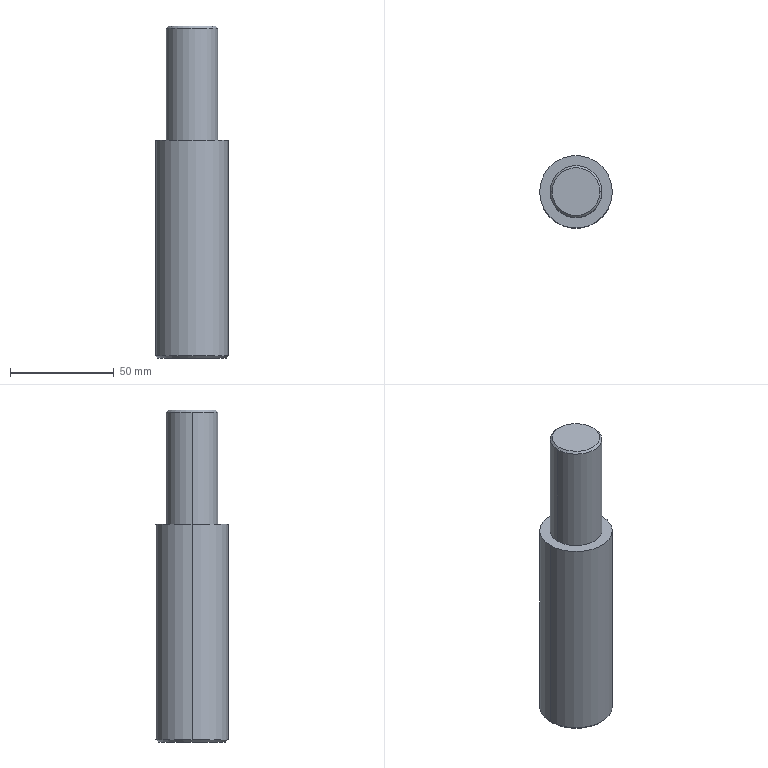Part | SolidWorks | features Chamfer 1, Extrusion 1, ICE 1 | 1 solid | 11 faces | box 35 x 35 x 160 mm | volume 127928 mm3 | cone 4 | cylinder 4 | plane 3 | commonest cylinder face diameters 25 x2 35 x2
STEP:
#1=CARTESIAN_POINT('',(11.5,0.,160.));
#2=VERTEX_POINT('',#1);
#3=CARTESIAN_POINT('',(-11.5,0.,160.));
#4=VERTEX_POINT('',#3);
#5=CARTESIAN_POINT('',(0.,0.,160.));
#6=DIRECTION('',(0.,0.,1.));
#7=DIRECTION('',(1.,0.,0.));
#8=AXIS2_PLACEMENT_3D('',#5,#6,#7);
#9=CIRCLE('',#8,11.5);
#10=EDGE_CURVE('',#2,#4,#9,.T.);
#11=ORIENTED_EDGE('',*,*,#10,.F.);
#12=CARTESIAN_POINT('',(12.5,0.,159.));
#13=VERTEX_POINT('',#12);
#14=CARTESIAN_POINT('',(11.5,0.,160.));
#15=DIRECTION('',(0.7071,0.,-0.7071));
#16=VECTOR('',#15,1000.);
#17=LINE('',#14,#16);
#18=EDGE_CURVE('',#2,#13,#17,.T.);
#19=ORIENTED_EDGE('',*,*,#18,.T.);
#20=CARTESIAN_POINT('',(-12.5,0.,159.));
#21=VERTEX_POINT('',#20);
#22=CARTESIAN_POINT('',(0.,0.,159.));
#23=DIRECTION('',(0.,0.,-1.));
#24=DIRECTION('',(1.,0.,0.));
#25=AXIS2_PLACEMENT_3D('',#22,#23,#24);
#26=CIRCLE('',#25,12.5);
#27=EDGE_CURVE('',#21,#13,#26,.T.);
#28=ORIENTED_EDGE('',*,*,#27,.F.);
#29=CARTESIAN_POINT('',(-11.5,0.,160.));
#30=DIRECTION('',(-0.7071,0.,-0.7071));
#31=VECTOR('',#30,1000.);
#32=LINE('',#29,#31);
#33=EDGE_CURVE('',#4,#21,#32,.T.);
#34=ORIENTED_EDGE('',*,*,#33,.F.);
#35=EDGE_LOOP('',(#11,#19,#28,#34));
#36=FACE_OUTER_BOUND('',#35,.T.);
#37=CARTESIAN_POINT('',(0.,0.,160.));
#38=DIRECTION('',(0.,0.,-1.));
#39=DIRECTION('',(-1.,0.,0.));
#40=AXIS2_PLACEMENT_3D('',#37,#38,#39);
#41=CONICAL_SURFACE('',#40,11.5,0.7854);
#42=ADVANCED_FACE('',(#36),#41,.T.);
#43=CARTESIAN_POINT('',(-16.5,0.,0.));
#44=VERTEX_POINT('',#43);
#45=CARTESIAN_POINT('',(16.5,0.,0.));
#46=VERTEX_POINT('',#45);
#47=CARTESIAN_POINT('',(0.,0.,0.));
#48=DIRECTION('',(0.,0.,-1.));
#49=DIRECTION('',(1.,0.,0.));
#50=AXIS2_PLACEMENT_3D('',#47,#48,#49);
#51=CIRCLE('',#50,16.5);
#52=EDGE_CURVE('',#44,#46,#51,.T.);
#53=ORIENTED_EDGE('',*,*,#52,.F.);
#54=CARTESIAN_POINT('',(-17.5,0.,1.));
#55=VERTEX_POINT('',#54);
#56=CARTESIAN_POINT('',(-17.5,0.,1.));
#57=DIRECTION('',(-0.7071,0.,0.7071));
#58=VECTOR('',#57,1000.);
#59=LINE('',#56,#58);
#60=EDGE_CURVE('',#44,#55,#59,.T.);
#61=ORIENTED_EDGE('',*,*,#60,.T.);
#62=CARTESIAN_POINT('',(17.5,0.,1.));
#63=VERTEX_POINT('',#62);
#64=CARTESIAN_POINT('',(0.,0.,1.));
#65=DIRECTION('',(0.,0.,1.));
#66=DIRECTION('',(1.,0.,0.));
#67=AXIS2_PLACEMENT_3D('',#64,#65,#66);
#68=CIRCLE('',#67,17.5);
#69=EDGE_CURVE('',#63,#55,#68,.T.);
#70=ORIENTED_EDGE('',*,*,#69,.F.);
#71=CARTESIAN_POINT('',(17.5,0.,1.));
#72=DIRECTION('',(0.7071,0.,0.7071));
#73=VECTOR('',#72,1000.);
#74=LINE('',#71,#73);
#75=EDGE_CURVE('',#46,#63,#74,.T.);
#76=ORIENTED_EDGE('',*,*,#75,.F.);
#77=EDGE_LOOP('',(#53,#61,#70,#76));
#78=FACE_OUTER_BOUND('',#77,.T.);
#79=CARTESIAN_POINT('',(0.,0.,1.));
#80=DIRECTION('',(0.,0.,1.));
#81=DIRECTION('',(1.,0.,0.));
#82=AXIS2_PLACEMENT_3D('',#79,#80,#81);
#83=CONICAL_SURFACE('',#82,17.5,0.7854);
#84=ADVANCED_FACE('',(#78),#83,.T.);
#85=ORIENTED_EDGE('',*,*,#27,.T.);
#86=CARTESIAN_POINT('',(12.5,0.,105.));
#87=VERTEX_POINT('',#86);
#88=CARTESIAN_POINT('',(12.5,0.,160.));
#89=DIRECTION('',(0.,0.,-1.));
#90=VECTOR('',#89,1000.);
#91=LINE('',#88,#90);
#92=EDGE_CURVE('',#13,#87,#91,.T.);
#93=ORIENTED_EDGE('',*,*,#92,.T.);
#94=CARTESIAN_POINT('',(-12.5,0.,105.));
#95=VERTEX_POINT('',#94);
#96=CARTESIAN_POINT('',(0.,0.,105.));
#97=DIRECTION('',(0.,0.,1.));
#98=DIRECTION('',(1.,0.,0.));
#99=AXIS2_PLACEMENT_3D('',#96,#97,#98);
#100=CIRCLE('',#99,12.5);
#101=EDGE_CURVE('',#87,#95,#100,.T.);
#102=ORIENTED_EDGE('',*,*,#101,.T.);
#103=CARTESIAN_POINT('',(-12.5,0.,160.));
#104=DIRECTION('',(0.,0.,-1.));
#105=VECTOR('',#104,1000.);
#106=LINE('',#103,#105);
#107=EDGE_CURVE('',#21,#95,#106,.T.);
#108=ORIENTED_EDGE('',*,*,#107,.F.);
#109=EDGE_LOOP('',(#85,#93,#102,#108));
#110=FACE_OUTER_BOUND('',#109,.T.);
#111=CARTESIAN_POINT('',(0.,0.,160.));
#112=DIRECTION('',(0.,0.,-1.));
#113=DIRECTION('',(-1.,0.,0.));
#114=AXIS2_PLACEMENT_3D('',#111,#112,#113);
#115=CYLINDRICAL_SURFACE('',#114,12.5);
#116=ADVANCED_FACE('',(#110),#115,.T.);
#117=CARTESIAN_POINT('',(17.5,0.,105.));
#118=VERTEX_POINT('',#117);
#119=CARTESIAN_POINT('',(-17.5,0.,105.));
#120=VERTEX_POINT('',#119);
#121=CARTESIAN_POINT('',(0.,0.,105.));
#122=DIRECTION('',(0.,0.,1.));
#123=DIRECTION('',(1.,0.,0.));
#124=AXIS2_PLACEMENT_3D('',#121,#122,#123);
#125=CIRCLE('',#124,17.5);
#126=EDGE_CURVE('',#118,#120,#125,.T.);
#127=ORIENTED_EDGE('',*,*,#126,.F.);
#128=CARTESIAN_POINT('',(17.5,0.,105.));
#129=DIRECTION('',(0.,0.,-1.));
#130=VECTOR('',#129,1000.);
#131=LINE('',#128,#130);
#132=EDGE_CURVE('',#118,#63,#131,.T.);
#133=ORIENTED_EDGE('',*,*,#132,.T.);
#134=ORIENTED_EDGE('',*,*,#69,.T.);
#135=CARTESIAN_POINT('',(-17.5,0.,105.));
#136=DIRECTION('',(0.,0.,-1.));
#137=VECTOR('',#136,1000.);
#138=LINE('',#135,#137);
#139=EDGE_CURVE('',#120,#55,#138,.T.);
#140=ORIENTED_EDGE('',*,*,#139,.F.);
#141=EDGE_LOOP('',(#127,#133,#134,#140));
#142=FACE_OUTER_BOUND('',#141,.T.);
#143=CARTESIAN_POINT('',(0.,0.,105.));
#144=DIRECTION('',(0.,0.,-1.));
#145=DIRECTION('',(-1.,0.,0.));
#146=AXIS2_PLACEMENT_3D('',#143,#144,#145);
#147=CYLINDRICAL_SURFACE('',#146,17.5);
#148=ADVANCED_FACE('',(#142),#147,.T.);
#149=ORIENTED_EDGE('',*,*,#132,.F.);
#150=CARTESIAN_POINT('',(0.,0.,105.));
#151=DIRECTION('',(0.,0.,1.));
#152=DIRECTION('',(1.,0.,0.));
#153=AXIS2_PLACEMENT_3D('',#150,#151,#152);
#154=CIRCLE('',#153,17.5);
#155=EDGE_CURVE('',#120,#118,#154,.T.);
#156=ORIENTED_EDGE('',*,*,#155,.F.);
#157=ORIENTED_EDGE('',*,*,#139,.T.);
#158=CARTESIAN_POINT('',(0.,0.,1.));
#159=DIRECTION('',(0.,0.,1.));
#160=DIRECTION('',(1.,0.,0.));
#161=AXIS2_PLACEMENT_3D('',#158,#159,#160);
#162=CIRCLE('',#161,17.5);
#163=EDGE_CURVE('',#55,#63,#162,.T.);
#164=ORIENTED_EDGE('',*,*,#163,.T.);
#165=EDGE_LOOP('',(#149,#156,#157,#164));
#166=FACE_OUTER_BOUND('',#165,.T.);
#167=CARTESIAN_POINT('',(0.,0.,105.));
#168=DIRECTION('',(0.,0.,-1.));
#169=DIRECTION('',(-1.,0.,0.));
#170=AXIS2_PLACEMENT_3D('',#167,#168,#169);
#171=CYLINDRICAL_SURFACE('',#170,17.5);
#172=ADVANCED_FACE('',(#166),#171,.T.);
#173=CARTESIAN_POINT('',(0.,0.,105.));
#174=DIRECTION('',(0.,0.,1.));
#175=DIRECTION('',(1.,0.,0.));
#176=AXIS2_PLACEMENT_3D('',#173,#174,#175);
#177=CIRCLE('',#176,12.5);
#178=EDGE_CURVE('',#95,#87,#177,.T.);
#179=ORIENTED_EDGE('',*,*,#178,.F.);
#180=ORIENTED_EDGE('',*,*,#101,.F.);
#181=EDGE_LOOP('',(#179,#180));
#182=FACE_BOUND('',#181,.T.);
#183=ORIENTED_EDGE('',*,*,#155,.T.);
#184=ORIENTED_EDGE('',*,*,#126,.T.);
#185=EDGE_LOOP('',(#183,#184));
#186=FACE_OUTER_BOUND('',#185,.T.);
#187=CARTESIAN_POINT('',(0.,0.,105.));
#188=DIRECTION('',(0.,0.,1.));
#189=DIRECTION('',(1.,0.,0.));
#190=AXIS2_PLACEMENT_3D('',#187,#188,#189);
#191=PLANE('',#190);
#192=ADVANCED_FACE('',(#182,#186),#191,.T.);
#193=CARTESIAN_POINT('',(0.,0.,0.));
#194=DIRECTION('',(0.,0.,-1.));
#195=DIRECTION('',(1.,0.,0.));
#196=AXIS2_PLACEMENT_3D('',#193,#194,#195);
#197=CIRCLE('',#196,16.5);
#198=EDGE_CURVE('',#46,#44,#197,.T.);
#199=ORIENTED_EDGE('',*,*,#198,.T.);
#200=ORIENTED_EDGE('',*,*,#52,.T.);
#201=EDGE_LOOP('',(#199,#200));
#202=FACE_OUTER_BOUND('',#201,.T.);
#203=CARTESIAN_POINT('',(0.,0.,0.));
#204=DIRECTION('',(0.,0.,1.));
#205=DIRECTION('',(1.,0.,0.));
#206=AXIS2_PLACEMENT_3D('',#203,#204,#205);
#207=PLANE('',#206);
#208=ADVANCED_FACE('',(#202),#207,.F.);
#209=ORIENTED_EDGE('',*,*,#92,.F.);
#210=CARTESIAN_POINT('',(0.,0.,159.));
#211=DIRECTION('',(0.,0.,-1.));
#212=DIRECTION('',(1.,0.,0.));
#213=AXIS2_PLACEMENT_3D('',#210,#211,#212);
#214=CIRCLE('',#213,12.5);
#215=EDGE_CURVE('',#13,#21,#214,.T.);
#216=ORIENTED_EDGE('',*,*,#215,.T.);
#217=ORIENTED_EDGE('',*,*,#107,.T.);
#218=ORIENTED_EDGE('',*,*,#178,.T.);
#219=EDGE_LOOP('',(#209,#216,#217,#218));
#220=FACE_OUTER_BOUND('',#219,.T.);
#221=CARTESIAN_POINT('',(0.,0.,160.));
#222=DIRECTION('',(0.,0.,-1.));
#223=DIRECTION('',(-1.,0.,0.));
#224=AXIS2_PLACEMENT_3D('',#221,#222,#223);
#225=CYLINDRICAL_SURFACE('',#224,12.5);
#226=ADVANCED_FACE('',(#220),#225,.T.);
#227=CARTESIAN_POINT('',(0.,0.,160.));
#228=DIRECTION('',(0.,0.,1.));
#229=DIRECTION('',(1.,0.,0.));
#230=AXIS2_PLACEMENT_3D('',#227,#228,#229);
#231=CIRCLE('',#230,11.5);
#232=EDGE_CURVE('',#4,#2,#231,.T.);
#233=ORIENTED_EDGE('',*,*,#232,.T.);
#234=ORIENTED_EDGE('',*,*,#10,.T.);
#235=EDGE_LOOP('',(#233,#234));
#236=FACE_OUTER_BOUND('',#235,.T.);
#237=CARTESIAN_POINT('',(0.,0.,160.));
#238=DIRECTION('',(0.,0.,1.));
#239=DIRECTION('',(1.,0.,0.));
#240=AXIS2_PLACEMENT_3D('',#237,#238,#239);
#241=PLANE('',#240);
#242=ADVANCED_FACE('',(#236),#241,.T.);
#243=ORIENTED_EDGE('',*,*,#60,.F.);
#244=ORIENTED_EDGE('',*,*,#198,.F.);
#245=ORIENTED_EDGE('',*,*,#75,.T.);
#246=ORIENTED_EDGE('',*,*,#163,.F.);
#247=EDGE_LOOP('',(#243,#244,#245,#246));
#248=FACE_OUTER_BOUND('',#247,.T.);
#249=CARTESIAN_POINT('',(0.,0.,1.));
#250=DIRECTION('',(0.,0.,1.));
#251=DIRECTION('',(1.,0.,0.));
#252=AXIS2_PLACEMENT_3D('',#249,#250,#251);
#253=CONICAL_SURFACE('',#252,17.5,0.7854);
#254=ADVANCED_FACE('',(#248),#253,.T.);
#255=ORIENTED_EDGE('',*,*,#18,.F.);
#256=ORIENTED_EDGE('',*,*,#232,.F.);
#257=ORIENTED_EDGE('',*,*,#33,.T.);
#258=ORIENTED_EDGE('',*,*,#215,.F.);
#259=EDGE_LOOP('',(#255,#256,#257,#258));
#260=FACE_OUTER_BOUND('',#259,.T.);
#261=CARTESIAN_POINT('',(0.,0.,160.));
#262=DIRECTION('',(0.,0.,-1.));
#263=DIRECTION('',(-1.,0.,0.));
#264=AXIS2_PLACEMENT_3D('',#261,#262,#263);
#265=CONICAL_SURFACE('',#264,11.5,0.7854);
#266=ADVANCED_FACE('',(#260),#265,.T.);
#267=CLOSED_SHELL('',(#42,#84,#116,#148,#172,#192,#208,#226,#242,#254,#266));
#268=MANIFOLD_SOLID_BREP('',#267);
#269=CARTESIAN_POINT('',(0.,0.,0.));
#270=DIRECTION('',(0.,0.,1.));
#271=DIRECTION('',(1.,0.,0.));
#272=AXIS2_PLACEMENT_3D('',#269,#270,#271);
#273=(LENGTH_UNIT()NAMED_UNIT(*)SI_UNIT(.MILLI.,.METRE.));
#274=UNCERTAINTY_MEASURE_WITH_UNIT(LENGTH_MEASURE(0.00001),#273,'','');
#275=(NAMED_UNIT(*)PLANE_ANGLE_UNIT()SI_UNIT($,.RADIAN.));
#276=(NAMED_UNIT(*)SI_UNIT($,.STERADIAN.)SOLID_ANGLE_UNIT());
#277=(GEOMETRIC_REPRESENTATION_CONTEXT(3)GLOBAL_UNCERTAINTY_ASSIGNED_CONTEXT((#274))GLOBAL_UNIT_ASSIGNED_CONTEXT((#273,#275,#276))REPRESENTATION_CONTEXT('',''));
#278=ADVANCED_BREP_SHAPE_REPRESENTATION('',(#268,#272),#277);